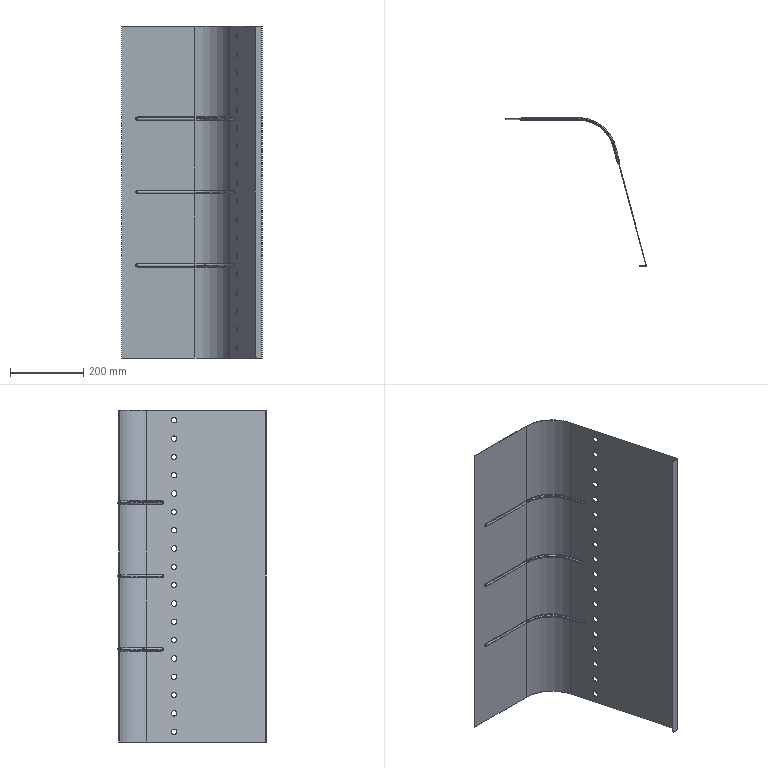Part | STEP file | 750078463 | 4 solids | 162 faces | box 383.962 x 404.825 x 906 mm | volume 774801 mm3 | cylinder 98 | spline 54 | plane 10 | commonest cylinder face diameters 15 x36 6 x18 2 x12 4.4 x12 8.4 x6 197.6 x4